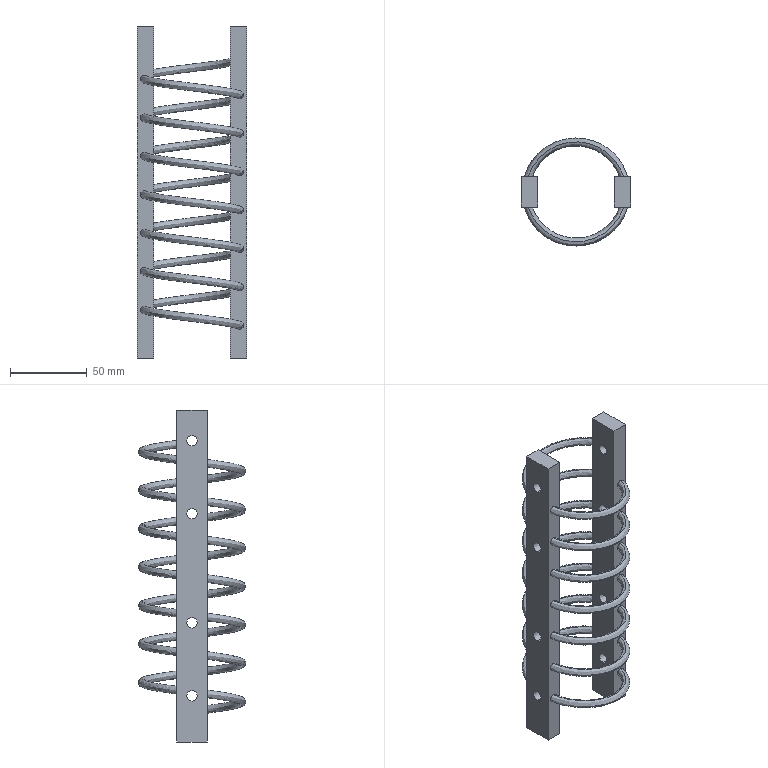Part | SolidWorks | features BaseBody 1, ICE 1 | 1 solid | 56 faces | box 71 x 70 x 216 mm | volume 111132 mm3 | spline 28 | cylinder 16 | plane 12 | commonest cylinder face diameters 6.8 x16